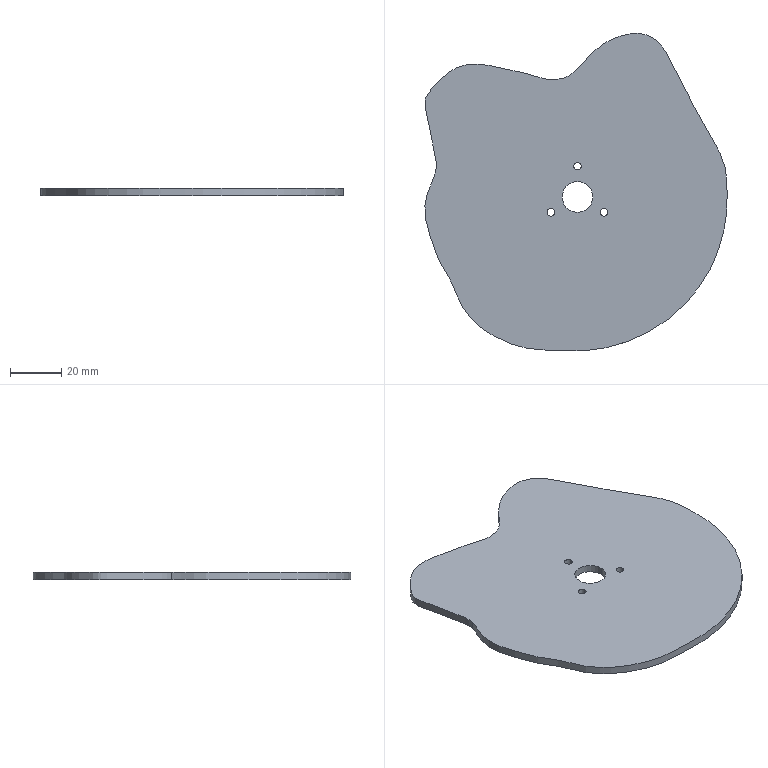Part | SolidWorks | features CurveInFile 1, Extrusion 1, ICE 1 | 1 solid | 12 faces | box 118.036 x 124.021 x 3 mm | volume 33767 mm3 | cylinder 8 | spline 2 | plane 2 | commonest cylinder face diameters 3 x6 12 x2